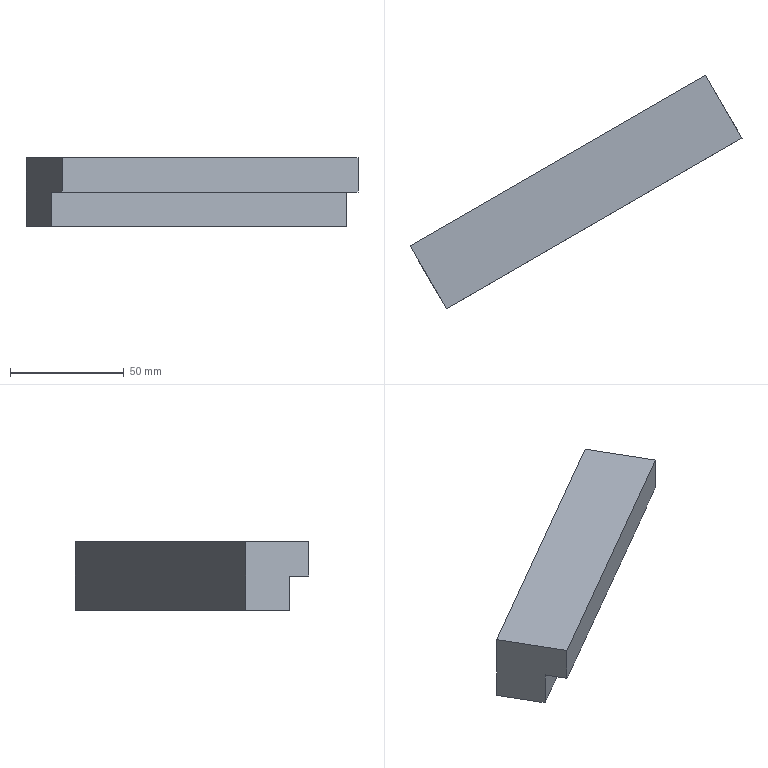Part | NX | features solid 2 | 1 solid | 8 faces | box 145.904 x 102.713 x 30 mm | volume 121500 mm3 | plane 8
STEP:
#1=CARTESIAN_POINT('',(-868.708,242.479,-110.));
#2=VERTEX_POINT('',#1);
#3=CARTESIAN_POINT('',(-868.708,242.479,-140.));
#4=VERTEX_POINT('',#3);
#5=CARTESIAN_POINT('',(-868.708,242.479,-125.));
#6=DIRECTION('',(0.,0.,-1.));
#7=VECTOR('',#6,1000.);
#8=LINE('',#5,#7);
#9=EDGE_CURVE('',#2,#4,#8,.T.);
#10=ORIENTED_EDGE('',*,*,#9,.T.);
#11=CARTESIAN_POINT('',(-857.708,223.426,-140.));
#12=VERTEX_POINT('',#11);
#13=CARTESIAN_POINT('',(-774.208,78.8,-140.));
#14=DIRECTION('',(0.5,-0.866,0.));
#15=VECTOR('',#14,1000.);
#16=LINE('',#13,#15);
#17=EDGE_CURVE('',#4,#12,#16,.T.);
#18=ORIENTED_EDGE('',*,*,#17,.T.);
#19=CARTESIAN_POINT('',(-857.708,223.426,-125.));
#20=VERTEX_POINT('',#19);
#21=CARTESIAN_POINT('',(-857.708,223.426,-125.));
#22=DIRECTION('',(0.,0.,-1.));
#23=VECTOR('',#22,1000.);
#24=LINE('',#21,#23);
#25=EDGE_CURVE('',#20,#12,#24,.T.);
#26=ORIENTED_EDGE('',*,*,#25,.F.);
#27=CARTESIAN_POINT('',(-852.708,214.766,-125.));
#28=VERTEX_POINT('',#27);
#29=CARTESIAN_POINT('',(-774.208,78.8,-125.));
#30=DIRECTION('',(-0.5,0.866,0.));
#31=VECTOR('',#30,1000.);
#32=LINE('',#29,#31);
#33=EDGE_CURVE('',#28,#20,#32,.T.);
#34=ORIENTED_EDGE('',*,*,#33,.F.);
#35=CARTESIAN_POINT('',(-852.708,214.766,-110.));
#36=VERTEX_POINT('',#35);
#37=CARTESIAN_POINT('',(-852.708,214.766,-125.));
#38=DIRECTION('',(0.,0.,1.));
#39=VECTOR('',#38,1000.);
#40=LINE('',#37,#39);
#41=EDGE_CURVE('',#28,#36,#40,.T.);
#42=ORIENTED_EDGE('',*,*,#41,.T.);
#43=CARTESIAN_POINT('',(-857.708,223.426,-110.));
#44=DIRECTION('',(0.5,-0.866,0.));
#45=VECTOR('',#44,1000.);
#46=LINE('',#43,#45);
#47=EDGE_CURVE('',#36,#2,#46,.F.);
#48=ORIENTED_EDGE('',*,*,#47,.T.);
#49=EDGE_LOOP('',(#10,#18,#26,#34,#42,#48));
#50=FACE_BOUND('',#49,.T.);
#51=CARTESIAN_POINT('',(-774.208,78.8,-125.));
#52=DIRECTION('',(0.866,0.5,0.));
#53=DIRECTION('',(0.,0.,-1.));
#54=AXIS2_PLACEMENT_3D('',#51,#52,#53);
#55=PLANE('',#54);
#56=ADVANCED_FACE('',(#50),#55,.F.);
#57=ORIENTED_EDGE('',*,*,#17,.F.);
#58=CARTESIAN_POINT('',(-738.804,317.479,-140.));
#59=VERTEX_POINT('',#58);
#60=CARTESIAN_POINT('',(-872.505,240.286,-140.));
#61=DIRECTION('',(0.866,0.5,0.));
#62=VECTOR('',#61,1000.);
#63=LINE('',#60,#62);
#64=EDGE_CURVE('',#4,#59,#63,.T.);
#65=ORIENTED_EDGE('',*,*,#64,.T.);
#66=CARTESIAN_POINT('',(-727.804,298.426,-140.));
#67=VERTEX_POINT('',#66);
#68=CARTESIAN_POINT('',(-738.804,317.479,-140.));
#69=DIRECTION('',(-0.5,0.866,0.));
#70=VECTOR('',#69,1000.);
#71=LINE('',#68,#70);
#72=EDGE_CURVE('',#59,#67,#71,.F.);
#73=ORIENTED_EDGE('',*,*,#72,.T.);
#74=CARTESIAN_POINT('',(-861.505,221.234,-140.));
#75=DIRECTION('',(-0.866,-0.5,0.));
#76=VECTOR('',#75,1000.);
#77=LINE('',#74,#76);
#78=EDGE_CURVE('',#12,#67,#77,.F.);
#79=ORIENTED_EDGE('',*,*,#78,.F.);
#80=EDGE_LOOP('',(#57,#65,#73,#79));
#81=FACE_BOUND('',#80,.T.);
#82=CARTESIAN_POINT('',(-872.505,240.286,-140.));
#83=DIRECTION('',(0.,0.,1.));
#84=DIRECTION('',(0.866,0.5,0.));
#85=AXIS2_PLACEMENT_3D('',#82,#83,#84);
#86=PLANE('',#85);
#87=ADVANCED_FACE('',(#81),#86,.F.);
#88=CARTESIAN_POINT('',(-738.804,317.479,-110.));
#89=VERTEX_POINT('',#88);
#90=CARTESIAN_POINT('',(-738.804,317.479,-125.));
#91=DIRECTION('',(0.,0.,1.));
#92=VECTOR('',#91,1000.);
#93=LINE('',#90,#92);
#94=EDGE_CURVE('',#89,#59,#93,.F.);
#95=ORIENTED_EDGE('',*,*,#94,.F.);
#96=CARTESIAN_POINT('',(-722.804,289.766,-110.));
#97=VERTEX_POINT('',#96);
#98=CARTESIAN_POINT('',(-730.097,302.398,-110.));
#99=DIRECTION('',(-0.5,0.866,0.));
#100=VECTOR('',#99,1000.);
#101=LINE('',#98,#100);
#102=EDGE_CURVE('',#97,#89,#101,.T.);
#103=ORIENTED_EDGE('',*,*,#102,.F.);
#104=CARTESIAN_POINT('',(-722.804,289.766,-125.));
#105=VERTEX_POINT('',#104);
#106=CARTESIAN_POINT('',(-722.804,289.766,-125.));
#107=DIRECTION('',(0.,0.,-1.));
#108=VECTOR('',#107,1000.);
#109=LINE('',#106,#108);
#110=EDGE_CURVE('',#105,#97,#109,.F.);
#111=ORIENTED_EDGE('',*,*,#110,.F.);
#112=CARTESIAN_POINT('',(-727.804,298.426,-125.));
#113=VERTEX_POINT('',#112);
#114=CARTESIAN_POINT('',(-727.804,298.426,-125.));
#115=DIRECTION('',(0.5,-0.866,0.));
#116=VECTOR('',#115,1000.);
#117=LINE('',#114,#116);
#118=EDGE_CURVE('',#105,#113,#117,.F.);
#119=ORIENTED_EDGE('',*,*,#118,.T.);
#120=CARTESIAN_POINT('',(-727.804,298.426,-125.));
#121=DIRECTION('',(0.,0.,1.));
#122=VECTOR('',#121,1000.);
#123=LINE('',#120,#122);
#124=EDGE_CURVE('',#113,#67,#123,.F.);
#125=ORIENTED_EDGE('',*,*,#124,.T.);
#126=ORIENTED_EDGE('',*,*,#72,.F.);
#127=EDGE_LOOP('',(#95,#103,#111,#119,#125,#126));
#128=FACE_BOUND('',#127,.T.);
#129=CARTESIAN_POINT('',(-730.097,302.398,-129.));
#130=DIRECTION('',(0.866,0.5,0.));
#131=DIRECTION('',(0.5,-0.866,0.));
#132=AXIS2_PLACEMENT_3D('',#129,#130,#131);
#133=PLANE('',#132);
#134=ADVANCED_FACE('',(#128),#133,.T.);
#135=ORIENTED_EDGE('',*,*,#78,.T.);
#136=ORIENTED_EDGE('',*,*,#124,.F.);
#137=CARTESIAN_POINT('',(-861.505,221.234,-125.));
#138=DIRECTION('',(-0.866,-0.5,0.));
#139=VECTOR('',#138,1000.);
#140=LINE('',#137,#139);
#141=EDGE_CURVE('',#20,#113,#140,.F.);
#142=ORIENTED_EDGE('',*,*,#141,.F.);
#143=ORIENTED_EDGE('',*,*,#25,.T.);
#144=EDGE_LOOP('',(#135,#136,#142,#143));
#145=FACE_BOUND('',#144,.T.);
#146=CARTESIAN_POINT('',(-861.505,221.234,-125.));
#147=DIRECTION('',(0.5,-0.866,0.));
#148=DIRECTION('',(-0.866,-0.5,0.));
#149=AXIS2_PLACEMENT_3D('',#146,#147,#148);
#150=PLANE('',#149);
#151=ADVANCED_FACE('',(#145),#150,.T.);
#152=ORIENTED_EDGE('',*,*,#64,.F.);
#153=ORIENTED_EDGE('',*,*,#9,.F.);
#154=CARTESIAN_POINT('',(-872.505,240.286,-110.));
#155=DIRECTION('',(0.866,0.5,0.));
#156=VECTOR('',#155,1000.);
#157=LINE('',#154,#156);
#158=EDGE_CURVE('',#2,#89,#157,.T.);
#159=ORIENTED_EDGE('',*,*,#158,.T.);
#160=ORIENTED_EDGE('',*,*,#94,.T.);
#161=EDGE_LOOP('',(#152,#153,#159,#160));
#162=FACE_BOUND('',#161,.T.);
#163=CARTESIAN_POINT('',(-872.505,240.286,-125.));
#164=DIRECTION('',(0.5,-0.866,0.));
#165=DIRECTION('',(-0.866,-0.5,0.));
#166=AXIS2_PLACEMENT_3D('',#163,#164,#165);
#167=PLANE('',#166);
#168=ADVANCED_FACE('',(#162),#167,.F.);
#169=ORIENTED_EDGE('',*,*,#141,.T.);
#170=ORIENTED_EDGE('',*,*,#118,.F.);
#171=CARTESIAN_POINT('',(-856.505,212.574,-125.));
#172=DIRECTION('',(0.866,0.5,0.));
#173=VECTOR('',#172,1000.);
#174=LINE('',#171,#173);
#175=EDGE_CURVE('',#28,#105,#174,.T.);
#176=ORIENTED_EDGE('',*,*,#175,.F.);
#177=ORIENTED_EDGE('',*,*,#33,.T.);
#178=EDGE_LOOP('',(#169,#170,#176,#177));
#179=FACE_BOUND('',#178,.T.);
#180=CARTESIAN_POINT('',(-861.505,221.234,-125.));
#181=DIRECTION('',(0.,0.,-1.));
#182=DIRECTION('',(0.866,0.5,0.));
#183=AXIS2_PLACEMENT_3D('',#180,#181,#182);
#184=PLANE('',#183);
#185=ADVANCED_FACE('',(#179),#184,.T.);
#186=ORIENTED_EDGE('',*,*,#102,.T.);
#187=ORIENTED_EDGE('',*,*,#158,.F.);
#188=ORIENTED_EDGE('',*,*,#47,.F.);
#189=CARTESIAN_POINT('',(-856.505,212.574,-110.));
#190=DIRECTION('',(0.866,0.5,0.));
#191=VECTOR('',#190,1000.);
#192=LINE('',#189,#191);
#193=EDGE_CURVE('',#36,#97,#192,.T.);
#194=ORIENTED_EDGE('',*,*,#193,.T.);
#195=EDGE_LOOP('',(#186,#187,#188,#194));
#196=FACE_BOUND('',#195,.T.);
#197=CARTESIAN_POINT('',(-861.505,221.234,-110.));
#198=DIRECTION('',(0.,0.,-1.));
#199=DIRECTION('',(0.866,0.5,0.));
#200=AXIS2_PLACEMENT_3D('',#197,#198,#199);
#201=PLANE('',#200);
#202=ADVANCED_FACE('',(#196),#201,.F.);
#203=ORIENTED_EDGE('',*,*,#193,.F.);
#204=ORIENTED_EDGE('',*,*,#41,.F.);
#205=ORIENTED_EDGE('',*,*,#175,.T.);
#206=ORIENTED_EDGE('',*,*,#110,.T.);
#207=EDGE_LOOP('',(#203,#204,#205,#206));
#208=FACE_BOUND('',#207,.T.);
#209=CARTESIAN_POINT('',(-856.505,212.574,-125.));
#210=DIRECTION('',(-0.5,0.866,0.));
#211=DIRECTION('',(0.866,0.5,0.));
#212=AXIS2_PLACEMENT_3D('',#209,#210,#211);
#213=PLANE('',#212);
#214=ADVANCED_FACE('',(#208),#213,.F.);
#215=CLOSED_SHELL('',(#56,#87,#134,#151,#168,#185,#202,#214));
#216=MANIFOLD_SOLID_BREP('',#215);
#217=(LENGTH_UNIT()NAMED_UNIT(*)SI_UNIT(.MILLI.,.METRE.));
#218=UNCERTAINTY_MEASURE_WITH_UNIT(LENGTH_MEASURE(0.00001),#217,'','');
#219=(NAMED_UNIT(*)PLANE_ANGLE_UNIT()SI_UNIT($,.RADIAN.));
#220=(NAMED_UNIT(*)SI_UNIT($,.STERADIAN.)SOLID_ANGLE_UNIT());
#221=(GEOMETRIC_REPRESENTATION_CONTEXT(3)GLOBAL_UNCERTAINTY_ASSIGNED_CONTEXT((#218))GLOBAL_UNIT_ASSIGNED_CONTEXT((#217,#219,#220))REPRESENTATION_CONTEXT('',''));
#222=ADVANCED_BREP_SHAPE_REPRESENTATION('',(#216),#221);